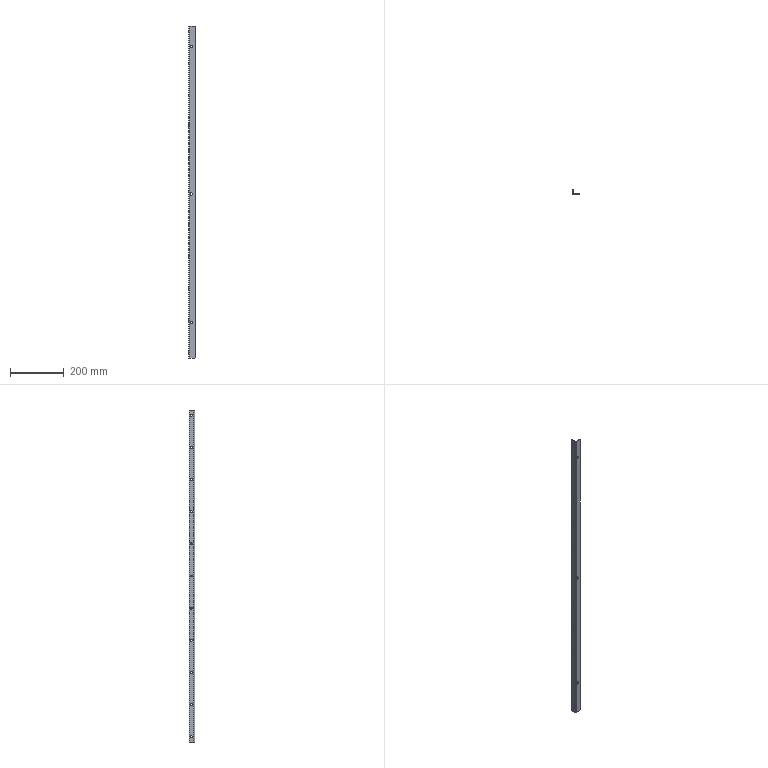Part | NX | features solid 2 | 1 solid | 40 faces | box 25 x 20 x 1240 mm | volume 102183 mm3 | cylinder 30 | plane 10 | commonest cylinder face diameters 7 x22 9.2 x6 4 x1 8 x1
STEP:
#1=CARTESIAN_POINT('',(652.,2.,1242.5));
#2=VERTEX_POINT('',#1);
#3=CARTESIAN_POINT('',(655.,2.,1239.5));
#4=VERTEX_POINT('',#3);
#5=CARTESIAN_POINT('',(655.,2.,1239.5));
#6=DIRECTION('',(0.7071,0.,-0.7071));
#7=VECTOR('',#6,1000.);
#8=LINE('',#5,#7);
#9=EDGE_CURVE('',#2,#4,#8,.T.);
#10=ORIENTED_EDGE('',*,*,#9,.F.);
#11=CARTESIAN_POINT('',(652.,0.,1242.5));
#12=VERTEX_POINT('',#11);
#13=CARTESIAN_POINT('',(652.,0.,1242.5));
#14=DIRECTION('',(0.,1.,0.));
#15=VECTOR('',#14,1000.);
#16=LINE('',#13,#15);
#17=EDGE_CURVE('',#12,#2,#16,.T.);
#18=ORIENTED_EDGE('',*,*,#17,.F.);
#19=CARTESIAN_POINT('',(655.,0.,1239.5));
#20=VERTEX_POINT('',#19);
#21=CARTESIAN_POINT('',(641.,0.,1253.5));
#22=DIRECTION('',(-0.7071,0.,0.7071));
#23=VECTOR('',#22,1000.);
#24=LINE('',#21,#23);
#25=EDGE_CURVE('',#20,#12,#24,.T.);
#26=ORIENTED_EDGE('',*,*,#25,.F.);
#27=CARTESIAN_POINT('',(655.,0.,1239.5));
#28=DIRECTION('',(0.,-1.,0.));
#29=VECTOR('',#28,1000.);
#30=LINE('',#27,#29);
#31=EDGE_CURVE('',#4,#20,#30,.T.);
#32=ORIENTED_EDGE('',*,*,#31,.F.);
#33=EDGE_LOOP('',(#10,#18,#26,#32));
#34=FACE_BOUND('',#33,.T.);
#35=CARTESIAN_POINT('',(655.,0.,1239.5));
#36=DIRECTION('',(-0.7071,0.,-0.7071));
#37=DIRECTION('',(-0.7071,0.,0.7071));
#38=AXIS2_PLACEMENT_3D('',#35,#36,#37);
#39=PLANE('',#38);
#40=ADVANCED_FACE('',(#34),#39,.F.);
#41=CARTESIAN_POINT('',(655.,2.,5.5));
#42=VERTEX_POINT('',#41);
#43=CARTESIAN_POINT('',(652.,2.,2.5));
#44=VERTEX_POINT('',#43);
#45=CARTESIAN_POINT('',(652.,2.,2.5));
#46=DIRECTION('',(-0.7071,0.,-0.7071));
#47=VECTOR('',#46,1000.);
#48=LINE('',#45,#47);
#49=EDGE_CURVE('',#42,#44,#48,.T.);
#50=ORIENTED_EDGE('',*,*,#49,.F.);
#51=CARTESIAN_POINT('',(655.,0.,5.5));
#52=VERTEX_POINT('',#51);
#53=CARTESIAN_POINT('',(655.,0.,5.5));
#54=DIRECTION('',(0.,1.,0.));
#55=VECTOR('',#54,1000.);
#56=LINE('',#53,#55);
#57=EDGE_CURVE('',#52,#42,#56,.T.);
#58=ORIENTED_EDGE('',*,*,#57,.F.);
#59=CARTESIAN_POINT('',(652.,0.,2.5));
#60=VERTEX_POINT('',#59);
#61=CARTESIAN_POINT('',(1261.,0.,611.5));
#62=DIRECTION('',(0.7071,0.,0.7071));
#63=VECTOR('',#62,1000.);
#64=LINE('',#61,#63);
#65=EDGE_CURVE('',#60,#52,#64,.T.);
#66=ORIENTED_EDGE('',*,*,#65,.F.);
#67=CARTESIAN_POINT('',(652.,0.,2.5));
#68=DIRECTION('',(0.,-1.,0.));
#69=VECTOR('',#68,1000.);
#70=LINE('',#67,#69);
#71=EDGE_CURVE('',#44,#60,#70,.T.);
#72=ORIENTED_EDGE('',*,*,#71,.F.);
#73=EDGE_LOOP('',(#50,#58,#66,#72));
#74=FACE_BOUND('',#73,.T.);
#75=CARTESIAN_POINT('',(652.,0.,2.5));
#76=DIRECTION('',(0.7071,0.,-0.7071));
#77=DIRECTION('',(0.,-1.,0.));
#78=AXIS2_PLACEMENT_3D('',#75,#76,#77);
#79=PLANE('',#78);
#80=ADVANCED_FACE('',(#74),#79,.T.);
#81=CARTESIAN_POINT('',(632.,9.,1222.5));
#82=VERTEX_POINT('',#81);
#83=CARTESIAN_POINT('',(630.,9.,1222.5));
#84=VERTEX_POINT('',#83);
#85=CARTESIAN_POINT('',(-608.413,9.,1222.5));
#86=DIRECTION('',(1.,0.,0.));
#87=VECTOR('',#86,1000.);
#88=LINE('',#85,#87);
#89=EDGE_CURVE('',#82,#84,#88,.F.);
#90=ORIENTED_EDGE('',*,*,#89,.T.);
#91=CARTESIAN_POINT('',(630.,16.,1222.5));
#92=VERTEX_POINT('',#91);
#93=CARTESIAN_POINT('',(630.,12.5,1222.5));
#94=DIRECTION('',(1.,0.,0.));
#95=DIRECTION('',(0.,1.,0.));
#96=AXIS2_PLACEMENT_3D('',#93,#94,#95);
#97=CIRCLE('',#96,3.5);
#98=EDGE_CURVE('',#92,#84,#97,.T.);
#99=ORIENTED_EDGE('',*,*,#98,.F.);
#100=CARTESIAN_POINT('',(632.,16.,1222.5));
#101=VERTEX_POINT('',#100);
#102=CARTESIAN_POINT('',(-608.413,16.,1222.5));
#103=DIRECTION('',(1.,0.,0.));
#104=VECTOR('',#103,1000.);
#105=LINE('',#102,#104);
#106=EDGE_CURVE('',#92,#101,#105,.T.);
#107=ORIENTED_EDGE('',*,*,#106,.T.);
#108=CARTESIAN_POINT('',(632.,12.5,1222.5));
#109=DIRECTION('',(1.,0.,0.));
#110=DIRECTION('',(0.,0.,-1.));
#111=AXIS2_PLACEMENT_3D('',#108,#109,#110);
#112=CIRCLE('',#111,3.5);
#113=EDGE_CURVE('',#101,#82,#112,.T.);
#114=ORIENTED_EDGE('',*,*,#113,.T.);
#115=EDGE_LOOP('',(#90,#99,#107,#114));
#116=FACE_BOUND('',#115,.T.);
#117=CARTESIAN_POINT('',(-608.413,12.5,1222.5));
#118=DIRECTION('',(1.,0.,0.));
#119=DIRECTION('',(0.,1.,0.));
#120=AXIS2_PLACEMENT_3D('',#117,#118,#119);
#121=CYLINDRICAL_SURFACE('',#120,3.5);
#122=ADVANCED_FACE('',(#116),#121,.F.);
#123=CARTESIAN_POINT('',(632.,9.,1102.5));
#124=VERTEX_POINT('',#123);
#125=CARTESIAN_POINT('',(630.,9.,1102.5));
#126=VERTEX_POINT('',#125);
#127=CARTESIAN_POINT('',(-608.413,9.,1102.5));
#128=DIRECTION('',(1.,0.,0.));
#129=VECTOR('',#128,1000.);
#130=LINE('',#127,#129);
#131=EDGE_CURVE('',#124,#126,#130,.F.);
#132=ORIENTED_EDGE('',*,*,#131,.T.);
#133=CARTESIAN_POINT('',(630.,16.,1102.5));
#134=VERTEX_POINT('',#133);
#135=CARTESIAN_POINT('',(630.,12.5,1102.5));
#136=DIRECTION('',(1.,0.,0.));
#137=DIRECTION('',(0.,1.,0.));
#138=AXIS2_PLACEMENT_3D('',#135,#136,#137);
#139=CIRCLE('',#138,3.5);
#140=EDGE_CURVE('',#134,#126,#139,.T.);
#141=ORIENTED_EDGE('',*,*,#140,.F.);
#142=CARTESIAN_POINT('',(632.,16.,1102.5));
#143=VERTEX_POINT('',#142);
#144=CARTESIAN_POINT('',(-608.413,16.,1102.5));
#145=DIRECTION('',(1.,0.,0.));
#146=VECTOR('',#145,1000.);
#147=LINE('',#144,#146);
#148=EDGE_CURVE('',#134,#143,#147,.T.);
#149=ORIENTED_EDGE('',*,*,#148,.T.);
#150=CARTESIAN_POINT('',(632.,12.5,1102.5));
#151=DIRECTION('',(1.,0.,0.));
#152=DIRECTION('',(0.,0.,-1.));
#153=AXIS2_PLACEMENT_3D('',#150,#151,#152);
#154=CIRCLE('',#153,3.5);
#155=EDGE_CURVE('',#143,#124,#154,.T.);
#156=ORIENTED_EDGE('',*,*,#155,.T.);
#157=EDGE_LOOP('',(#132,#141,#149,#156));
#158=FACE_BOUND('',#157,.T.);
#159=CARTESIAN_POINT('',(-608.413,12.5,1102.5));
#160=DIRECTION('',(1.,0.,0.));
#161=DIRECTION('',(0.,1.,0.));
#162=AXIS2_PLACEMENT_3D('',#159,#160,#161);
#163=CYLINDRICAL_SURFACE('',#162,3.5);
#164=ADVANCED_FACE('',(#158),#163,.F.);
#165=CARTESIAN_POINT('',(630.,9.,982.5));
#166=VERTEX_POINT('',#165);
#167=CARTESIAN_POINT('',(632.,9.,982.5));
#168=VERTEX_POINT('',#167);
#169=CARTESIAN_POINT('',(-608.413,9.,982.5));
#170=DIRECTION('',(1.,0.,0.));
#171=VECTOR('',#170,1000.);
#172=LINE('',#169,#171);
#173=EDGE_CURVE('',#166,#168,#172,.T.);
#174=ORIENTED_EDGE('',*,*,#173,.F.);
#175=CARTESIAN_POINT('',(630.,16.,982.5));
#176=VERTEX_POINT('',#175);
#177=CARTESIAN_POINT('',(630.,12.5,982.5));
#178=DIRECTION('',(1.,0.,0.));
#179=DIRECTION('',(0.,1.,0.));
#180=AXIS2_PLACEMENT_3D('',#177,#178,#179);
#181=CIRCLE('',#180,3.5);
#182=EDGE_CURVE('',#176,#166,#181,.T.);
#183=ORIENTED_EDGE('',*,*,#182,.F.);
#184=CARTESIAN_POINT('',(632.,16.,982.5));
#185=VERTEX_POINT('',#184);
#186=CARTESIAN_POINT('',(-608.413,16.,982.5));
#187=DIRECTION('',(1.,0.,0.));
#188=VECTOR('',#187,1000.);
#189=LINE('',#186,#188);
#190=EDGE_CURVE('',#185,#176,#189,.F.);
#191=ORIENTED_EDGE('',*,*,#190,.F.);
#192=CARTESIAN_POINT('',(632.,12.5,982.5));
#193=DIRECTION('',(1.,0.,0.));
#194=DIRECTION('',(0.,0.,-1.));
#195=AXIS2_PLACEMENT_3D('',#192,#193,#194);
#196=CIRCLE('',#195,3.5);
#197=EDGE_CURVE('',#185,#168,#196,.T.);
#198=ORIENTED_EDGE('',*,*,#197,.T.);
#199=EDGE_LOOP('',(#174,#183,#191,#198));
#200=FACE_BOUND('',#199,.T.);
#201=CARTESIAN_POINT('',(-608.413,12.5,982.5));
#202=DIRECTION('',(1.,0.,0.));
#203=DIRECTION('',(0.,1.,0.));
#204=AXIS2_PLACEMENT_3D('',#201,#202,#203);
#205=CYLINDRICAL_SURFACE('',#204,3.5);
#206=ADVANCED_FACE('',(#200),#205,.F.);
#207=CARTESIAN_POINT('',(632.,9.,22.5));
#208=VERTEX_POINT('',#207);
#209=CARTESIAN_POINT('',(630.,9.,22.5));
#210=VERTEX_POINT('',#209);
#211=CARTESIAN_POINT('',(-608.413,9.,22.5));
#212=DIRECTION('',(1.,0.,0.));
#213=VECTOR('',#212,1000.);
#214=LINE('',#211,#213);
#215=EDGE_CURVE('',#208,#210,#214,.F.);
#216=ORIENTED_EDGE('',*,*,#215,.T.);
#217=CARTESIAN_POINT('',(630.,16.,22.5));
#218=VERTEX_POINT('',#217);
#219=CARTESIAN_POINT('',(630.,12.5,22.5));
#220=DIRECTION('',(1.,0.,0.));
#221=DIRECTION('',(0.,1.,0.));
#222=AXIS2_PLACEMENT_3D('',#219,#220,#221);
#223=CIRCLE('',#222,3.5);
#224=EDGE_CURVE('',#218,#210,#223,.T.);
#225=ORIENTED_EDGE('',*,*,#224,.F.);
#226=CARTESIAN_POINT('',(632.,16.,22.5));
#227=VERTEX_POINT('',#226);
#228=CARTESIAN_POINT('',(-608.413,16.,22.5));
#229=DIRECTION('',(1.,0.,0.));
#230=VECTOR('',#229,1000.);
#231=LINE('',#228,#230);
#232=EDGE_CURVE('',#218,#227,#231,.T.);
#233=ORIENTED_EDGE('',*,*,#232,.T.);
#234=CARTESIAN_POINT('',(632.,12.5,22.5));
#235=DIRECTION('',(1.,0.,0.));
#236=DIRECTION('',(0.,0.,-1.));
#237=AXIS2_PLACEMENT_3D('',#234,#235,#236);
#238=CIRCLE('',#237,3.5);
#239=EDGE_CURVE('',#227,#208,#238,.T.);
#240=ORIENTED_EDGE('',*,*,#239,.T.);
#241=EDGE_LOOP('',(#216,#225,#233,#240));
#242=FACE_BOUND('',#241,.T.);
#243=CARTESIAN_POINT('',(-608.413,12.5,22.5));
#244=DIRECTION('',(1.,0.,0.));
#245=DIRECTION('',(0.,1.,0.));
#246=AXIS2_PLACEMENT_3D('',#243,#244,#245);
#247=CYLINDRICAL_SURFACE('',#246,3.5);
#248=ADVANCED_FACE('',(#242),#247,.F.);
#249=CARTESIAN_POINT('',(630.,9.,142.5));
#250=VERTEX_POINT('',#249);
#251=CARTESIAN_POINT('',(632.,9.,142.5));
#252=VERTEX_POINT('',#251);
#253=CARTESIAN_POINT('',(-608.413,9.,142.5));
#254=DIRECTION('',(1.,0.,0.));
#255=VECTOR('',#254,1000.);
#256=LINE('',#253,#255);
#257=EDGE_CURVE('',#250,#252,#256,.T.);
#258=ORIENTED_EDGE('',*,*,#257,.F.);
#259=CARTESIAN_POINT('',(630.,16.,142.5));
#260=VERTEX_POINT('',#259);
#261=CARTESIAN_POINT('',(630.,12.5,142.5));
#262=DIRECTION('',(1.,0.,0.));
#263=DIRECTION('',(0.,1.,0.));
#264=AXIS2_PLACEMENT_3D('',#261,#262,#263);
#265=CIRCLE('',#264,3.5);
#266=EDGE_CURVE('',#260,#250,#265,.T.);
#267=ORIENTED_EDGE('',*,*,#266,.F.);
#268=CARTESIAN_POINT('',(632.,16.,142.5));
#269=VERTEX_POINT('',#268);
#270=CARTESIAN_POINT('',(-608.413,16.,142.5));
#271=DIRECTION('',(1.,0.,0.));
#272=VECTOR('',#271,1000.);
#273=LINE('',#270,#272);
#274=EDGE_CURVE('',#269,#260,#273,.F.);
#275=ORIENTED_EDGE('',*,*,#274,.F.);
#276=CARTESIAN_POINT('',(632.,12.5,142.5));
#277=DIRECTION('',(1.,0.,0.));
#278=DIRECTION('',(0.,0.,-1.));
#279=AXIS2_PLACEMENT_3D('',#276,#277,#278);
#280=CIRCLE('',#279,3.5);
#281=EDGE_CURVE('',#269,#252,#280,.T.);
#282=ORIENTED_EDGE('',*,*,#281,.T.);
#283=EDGE_LOOP('',(#258,#267,#275,#282));
#284=FACE_BOUND('',#283,.T.);
#285=CARTESIAN_POINT('',(-608.413,12.5,142.5));
#286=DIRECTION('',(1.,0.,0.));
#287=DIRECTION('',(0.,1.,0.));
#288=AXIS2_PLACEMENT_3D('',#285,#286,#287);
#289=CYLINDRICAL_SURFACE('',#288,3.5);
#290=ADVANCED_FACE('',(#284),#289,.F.);
#291=CARTESIAN_POINT('',(632.,9.,862.5));
#292=VERTEX_POINT('',#291);
#293=CARTESIAN_POINT('',(630.,9.,862.5));
#294=VERTEX_POINT('',#293);
#295=CARTESIAN_POINT('',(-608.413,9.,862.5));
#296=DIRECTION('',(1.,0.,0.));
#297=VECTOR('',#296,1000.);
#298=LINE('',#295,#297);
#299=EDGE_CURVE('',#292,#294,#298,.F.);
#300=ORIENTED_EDGE('',*,*,#299,.T.);
#301=CARTESIAN_POINT('',(630.,16.,862.5));
#302=VERTEX_POINT('',#301);
#303=CARTESIAN_POINT('',(630.,12.5,862.5));
#304=DIRECTION('',(1.,0.,0.));
#305=DIRECTION('',(0.,1.,0.));
#306=AXIS2_PLACEMENT_3D('',#303,#304,#305);
#307=CIRCLE('',#306,3.5);
#308=EDGE_CURVE('',#302,#294,#307,.T.);
#309=ORIENTED_EDGE('',*,*,#308,.F.);
#310=CARTESIAN_POINT('',(632.,16.,862.5));
#311=VERTEX_POINT('',#310);
#312=CARTESIAN_POINT('',(-608.413,16.,862.5));
#313=DIRECTION('',(1.,0.,0.));
#314=VECTOR('',#313,1000.);
#315=LINE('',#312,#314);
#316=EDGE_CURVE('',#302,#311,#315,.T.);
#317=ORIENTED_EDGE('',*,*,#316,.T.);
#318=CARTESIAN_POINT('',(632.,12.5,862.5));
#319=DIRECTION('',(1.,0.,0.));
#320=DIRECTION('',(0.,0.,-1.));
#321=AXIS2_PLACEMENT_3D('',#318,#319,#320);
#322=CIRCLE('',#321,3.5);
#323=EDGE_CURVE('',#311,#292,#322,.T.);
#324=ORIENTED_EDGE('',*,*,#323,.T.);
#325=EDGE_LOOP('',(#300,#309,#317,#324));
#326=FACE_BOUND('',#325,.T.);
#327=CARTESIAN_POINT('',(-608.413,12.5,862.5));
#328=DIRECTION('',(1.,0.,0.));
#329=DIRECTION('',(0.,1.,0.));
#330=AXIS2_PLACEMENT_3D('',#327,#328,#329);
#331=CYLINDRICAL_SURFACE('',#330,3.5);
#332=ADVANCED_FACE('',(#326),#331,.F.);
#333=CARTESIAN_POINT('',(630.,9.,742.5));
#334=VERTEX_POINT('',#333);
#335=CARTESIAN_POINT('',(632.,9.,742.5));
#336=VERTEX_POINT('',#335);
#337=CARTESIAN_POINT('',(-608.413,9.,742.5));
#338=DIRECTION('',(1.,0.,0.));
#339=VECTOR('',#338,1000.);
#340=LINE('',#337,#339);
#341=EDGE_CURVE('',#334,#336,#340,.T.);
#342=ORIENTED_EDGE('',*,*,#341,.F.);
#343=CARTESIAN_POINT('',(630.,16.,742.5));
#344=VERTEX_POINT('',#343);
#345=CARTESIAN_POINT('',(630.,12.5,742.5));
#346=DIRECTION('',(1.,0.,0.));
#347=DIRECTION('',(0.,1.,0.));
#348=AXIS2_PLACEMENT_3D('',#345,#346,#347);
#349=CIRCLE('',#348,3.5);
#350=EDGE_CURVE('',#344,#334,#349,.T.);
#351=ORIENTED_EDGE('',*,*,#350,.F.);
#352=CARTESIAN_POINT('',(632.,16.,742.5));
#353=VERTEX_POINT('',#352);
#354=CARTESIAN_POINT('',(-608.413,16.,742.5));
#355=DIRECTION('',(1.,0.,0.));
#356=VECTOR('',#355,1000.);
#357=LINE('',#354,#356);
#358=EDGE_CURVE('',#353,#344,#357,.F.);
#359=ORIENTED_EDGE('',*,*,#358,.F.);
#360=CARTESIAN_POINT('',(632.,12.5,742.5));
#361=DIRECTION('',(1.,0.,0.));
#362=DIRECTION('',(0.,0.,-1.));
#363=AXIS2_PLACEMENT_3D('',#360,#361,#362);
#364=CIRCLE('',#363,3.5);
#365=EDGE_CURVE('',#353,#336,#364,.T.);
#366=ORIENTED_EDGE('',*,*,#365,.T.);
#367=EDGE_LOOP('',(#342,#351,#359,#366));
#368=FACE_BOUND('',#367,.T.);
#369=CARTESIAN_POINT('',(-608.413,12.5,742.5));
#370=DIRECTION('',(1.,0.,0.));
#371=DIRECTION('',(0.,1.,0.));
#372=AXIS2_PLACEMENT_3D('',#369,#370,#371);
#373=CYLINDRICAL_SURFACE('',#372,3.5);
#374=ADVANCED_FACE('',(#368),#373,.F.);
#375=CARTESIAN_POINT('',(632.,9.,622.5));
#376=VERTEX_POINT('',#375);
#377=CARTESIAN_POINT('',(630.,9.,622.5));
#378=VERTEX_POINT('',#377);
#379=CARTESIAN_POINT('',(-608.413,9.,622.5));
#380=DIRECTION('',(1.,0.,0.));
#381=VECTOR('',#380,1000.);
#382=LINE('',#379,#381);
#383=EDGE_CURVE('',#376,#378,#382,.F.);
#384=ORIENTED_EDGE('',*,*,#383,.T.);
#385=CARTESIAN_POINT('',(630.,16.,622.5));
#386=VERTEX_POINT('',#385);
#387=CARTESIAN_POINT('',(630.,12.5,622.5));
#388=DIRECTION('',(1.,0.,0.));
#389=DIRECTION('',(0.,1.,0.));
#390=AXIS2_PLACEMENT_3D('',#387,#388,#389);
#391=CIRCLE('',#390,3.5);
#392=EDGE_CURVE('',#386,#378,#391,.T.);
#393=ORIENTED_EDGE('',*,*,#392,.F.);
#394=CARTESIAN_POINT('',(632.,16.,622.5));
#395=VERTEX_POINT('',#394);
#396=CARTESIAN_POINT('',(-608.413,16.,622.5));
#397=DIRECTION('',(1.,0.,0.));
#398=VECTOR('',#397,1000.);
#399=LINE('',#396,#398);
#400=EDGE_CURVE('',#386,#395,#399,.T.);
#401=ORIENTED_EDGE('',*,*,#400,.T.);
#402=CARTESIAN_POINT('',(632.,12.5,622.5));
#403=DIRECTION('',(1.,0.,0.));
#404=DIRECTION('',(0.,0.,-1.));
#405=AXIS2_PLACEMENT_3D('',#402,#403,#404);
#406=CIRCLE('',#405,3.5);
#407=EDGE_CURVE('',#395,#376,#406,.T.);
#408=ORIENTED_EDGE('',*,*,#407,.T.);
#409=EDGE_LOOP('',(#384,#393,#401,#408));
#410=FACE_BOUND('',#409,.T.);
#411=CARTESIAN_POINT('',(-608.413,12.5,622.5));
#412=DIRECTION('',(1.,0.,0.));
#413=DIRECTION('',(0.,1.,0.));
#414=AXIS2_PLACEMENT_3D('',#411,#412,#413);
#415=CYLINDRICAL_SURFACE('',#414,3.5);
#416=ADVANCED_FACE('',(#410),#415,.F.);
#417=CARTESIAN_POINT('',(630.,9.,502.5));
#418=VERTEX_POINT('',#417);
#419=CARTESIAN_POINT('',(632.,9.,502.5));
#420=VERTEX_POINT('',#419);
#421=CARTESIAN_POINT('',(-608.413,9.,502.5));
#422=DIRECTION('',(1.,0.,0.));
#423=VECTOR('',#422,1000.);
#424=LINE('',#421,#423);
#425=EDGE_CURVE('',#418,#420,#424,.T.);
#426=ORIENTED_EDGE('',*,*,#425,.F.);
#427=CARTESIAN_POINT('',(630.,16.,502.5));
#428=VERTEX_POINT('',#427);
#429=CARTESIAN_POINT('',(630.,12.5,502.5));
#430=DIRECTION('',(1.,0.,0.));
#431=DIRECTION('',(0.,1.,0.));
#432=AXIS2_PLACEMENT_3D('',#429,#430,#431);
#433=CIRCLE('',#432,3.5);
#434=EDGE_CURVE('',#428,#418,#433,.T.);
#435=ORIENTED_EDGE('',*,*,#434,.F.);
#436=CARTESIAN_POINT('',(632.,16.,502.5));
#437=VERTEX_POINT('',#436);
#438=CARTESIAN_POINT('',(-608.413,16.,502.5));
#439=DIRECTION('',(1.,0.,0.));
#440=VECTOR('',#439,1000.);
#441=LINE('',#438,#440);
#442=EDGE_CURVE('',#437,#428,#441,.F.);
#443=ORIENTED_EDGE('',*,*,#442,.F.);
#444=CARTESIAN_POINT('',(632.,12.5,502.5));
#445=DIRECTION('',(1.,0.,0.));
#446=DIRECTION('',(0.,0.,-1.));
#447=AXIS2_PLACEMENT_3D('',#444,#445,#446);
#448=CIRCLE('',#447,3.5);
#449=EDGE_CURVE('',#437,#420,#448,.T.);
#450=ORIENTED_EDGE('',*,*,#449,.T.);
#451=EDGE_LOOP('',(#426,#435,#443,#450));
#452=FACE_BOUND('',#451,.T.);
#453=CARTESIAN_POINT('',(-608.413,12.5,502.5));
#454=DIRECTION('',(1.,0.,0.));
#455=DIRECTION('',(0.,1.,0.));
#456=AXIS2_PLACEMENT_3D('',#453,#454,#455);
#457=CYLINDRICAL_SURFACE('',#456,3.5);
#458=ADVANCED_FACE('',(#452),#457,.F.);
#459=CARTESIAN_POINT('',(630.,9.,382.5));
#460=VERTEX_POINT('',#459);
#461=CARTESIAN_POINT('',(632.,9.,382.5));
#462=VERTEX_POINT('',#461);
#463=CARTESIAN_POINT('',(-608.413,9.,382.5));
#464=DIRECTION('',(1.,0.,0.));
#465=VECTOR('',#464,1000.);
#466=LINE('',#463,#465);
#467=EDGE_CURVE('',#460,#462,#466,.T.);
#468=ORIENTED_EDGE('',*,*,#467,.F.);
#469=CARTESIAN_POINT('',(630.,16.,382.5));
#470=VERTEX_POINT('',#469);
#471=CARTESIAN_POINT('',(630.,12.5,382.5));
#472=DIRECTION('',(1.,0.,0.));
#473=DIRECTION('',(0.,1.,0.));
#474=AXIS2_PLACEMENT_3D('',#471,#472,#473);
#475=CIRCLE('',#474,3.5);
#476=EDGE_CURVE('',#470,#460,#475,.T.);
#477=ORIENTED_EDGE('',*,*,#476,.F.);
#478=CARTESIAN_POINT('',(632.,16.,382.5));
#479=VERTEX_POINT('',#478);
#480=CARTESIAN_POINT('',(-608.413,16.,382.5));
#481=DIRECTION('',(1.,0.,0.));
#482=VECTOR('',#481,1000.);
#483=LINE('',#480,#482);
#484=EDGE_CURVE('',#479,#470,#483,.F.);
#485=ORIENTED_EDGE('',*,*,#484,.F.);
#486=CARTESIAN_POINT('',(632.,12.5,382.5));
#487=DIRECTION('',(1.,0.,0.));
#488=DIRECTION('',(0.,0.,-1.));
#489=AXIS2_PLACEMENT_3D('',#486,#487,#488);
#490=CIRCLE('',#489,3.5);
#491=EDGE_CURVE('',#479,#462,#490,.T.);
#492=ORIENTED_EDGE('',*,*,#491,.T.);
#493=EDGE_LOOP('',(#468,#477,#485,#492));
#494=FACE_BOUND('',#493,.T.);
#495=CARTESIAN_POINT('',(-608.413,12.5,382.5));
#496=DIRECTION('',(1.,0.,0.));
#497=DIRECTION('',(0.,1.,0.));
#498=AXIS2_PLACEMENT_3D('',#495,#496,#497);
#499=CYLINDRICAL_SURFACE('',#498,3.5);
#500=ADVANCED_FACE('',(#494),#499,.F.);
#501=CARTESIAN_POINT('',(630.,9.,262.5));
#502=VERTEX_POINT('',#501);
#503=CARTESIAN_POINT('',(632.,9.,262.5));
#504=VERTEX_POINT('',#503);
#505=CARTESIAN_POINT('',(-608.413,9.,262.5));
#506=DIRECTION('',(1.,0.,0.));
#507=VECTOR('',#506,1000.);
#508=LINE('',#505,#507);
#509=EDGE_CURVE('',#502,#504,#508,.T.);
#510=ORIENTED_EDGE('',*,*,#509,.F.);
#511=CARTESIAN_POINT('',(630.,16.,262.5));
#512=VERTEX_POINT('',#511);
#513=CARTESIAN_POINT('',(630.,12.5,262.5));
#514=DIRECTION('',(1.,0.,0.));
#515=DIRECTION('',(0.,1.,0.));
#516=AXIS2_PLACEMENT_3D('',#513,#514,#515);
#517=CIRCLE('',#516,3.5);
#518=EDGE_CURVE('',#512,#502,#517,.T.);
#519=ORIENTED_EDGE('',*,*,#518,.F.);
#520=CARTESIAN_POINT('',(632.,16.,262.5));
#521=VERTEX_POINT('',#520);
#522=CARTESIAN_POINT('',(-608.413,16.,262.5));
#523=DIRECTION('',(1.,0.,0.));
#524=VECTOR('',#523,1000.);
#525=LINE('',#522,#524);
#526=EDGE_CURVE('',#521,#512,#525,.F.);
#527=ORIENTED_EDGE('',*,*,#526,.F.);
#528=CARTESIAN_POINT('',(632.,12.5,262.5));
#529=DIRECTION('',(1.,0.,0.));
#530=DIRECTION('',(0.,0.,-1.));
#531=AXIS2_PLACEMENT_3D('',#528,#529,#530);
#532=CIRCLE('',#531,3.5);
#533=EDGE_CURVE('',#521,#504,#532,.T.);
#534=ORIENTED_EDGE('',*,*,#533,.T.);
#535=EDGE_LOOP('',(#510,#519,#527,#534));
#536=FACE_BOUND('',#535,.T.);
#537=CARTESIAN_POINT('',(-608.413,12.5,262.5));
#538=DIRECTION('',(1.,0.,0.));
#539=DIRECTION('',(0.,1.,0.));
#540=AXIS2_PLACEMENT_3D('',#537,#538,#539);
#541=CYLINDRICAL_SURFACE('',#540,3.5);
#542=ADVANCED_FACE('',(#536),#541,.F.);
#543=CARTESIAN_POINT('',(640.,2.,619.6));
#544=VERTEX_POINT('',#543);
#545=CARTESIAN_POINT('',(640.,0.,619.6));
#546=VERTEX_POINT('',#545);
#547=CARTESIAN_POINT('',(640.,1240.413,619.6));
#548=DIRECTION('',(0.,-1.,0.));
#549=VECTOR('',#548,1000.);
#550=LINE('',#547,#549);
#551=EDGE_CURVE('',#544,#546,#550,.T.);
#552=ORIENTED_EDGE('',*,*,#551,.F.);
#553=CARTESIAN_POINT('',(640.,2.,610.4));
#554=VERTEX_POINT('',#553);
#555=CARTESIAN_POINT('',(640.,2.,615.));
#556=DIRECTION('',(0.,-1.,0.));
#557=DIRECTION('',(0.,0.,-1.));
#558=AXIS2_PLACEMENT_3D('',#555,#556,#557);
#559=CIRCLE('',#558,4.6);
#560=EDGE_CURVE('',#554,#544,#559,.T.);
#561=ORIENTED_EDGE('',*,*,#560,.F.);
#562=CARTESIAN_POINT('',(640.,0.,610.4));
#563=VERTEX_POINT('',#562);
#564=CARTESIAN_POINT('',(640.,1240.413,610.4));
#565=DIRECTION('',(0.,-1.,0.));
#566=VECTOR('',#565,1000.);
#567=LINE('',#564,#566);
#568=EDGE_CURVE('',#563,#554,#567,.F.);
#569=ORIENTED_EDGE('',*,*,#568,.F.);
#570=CARTESIAN_POINT('',(640.,0.,615.));
#571=DIRECTION('',(0.,-1.,0.));
#572=DIRECTION('',(0.,0.,1.));
#573=AXIS2_PLACEMENT_3D('',#570,#571,#572);
#574=CIRCLE('',#573,4.6);
#575=EDGE_CURVE('',#563,#546,#574,.T.);
#576=ORIENTED_EDGE('',*,*,#575,.T.);
#577=EDGE_LOOP('',(#552,#561,#569,#576));
#578=FACE_BOUND('',#577,.T.);
#579=CARTESIAN_POINT('',(640.,1240.413,615.));
#580=DIRECTION('',(0.,-1.,0.));
#581=DIRECTION('',(0.,0.,-1.));
#582=AXIS2_PLACEMENT_3D('',#579,#580,#581);
#583=CYLINDRICAL_SURFACE('',#582,4.6);
#584=ADVANCED_FACE('',(#578),#583,.F.);
#585=CARTESIAN_POINT('',(640.,2.,1169.6));
#586=VERTEX_POINT('',#585);
#587=CARTESIAN_POINT('',(640.,0.,1169.6));
#588=VERTEX_POINT('',#587);
#589=CARTESIAN_POINT('',(640.,1240.413,1169.6));
#590=DIRECTION('',(0.,-1.,0.));
#591=VECTOR('',#590,1000.);
#592=LINE('',#589,#591);
#593=EDGE_CURVE('',#586,#588,#592,.T.);
#594=ORIENTED_EDGE('',*,*,#593,.F.);
#595=CARTESIAN_POINT('',(640.,2.,1160.4));
#596=VERTEX_POINT('',#595);
#597=CARTESIAN_POINT('',(640.,2.,1165.));
#598=DIRECTION('',(0.,-1.,0.));
#599=DIRECTION('',(0.,0.,-1.));
#600=AXIS2_PLACEMENT_3D('',#597,#598,#599);
#601=CIRCLE('',#600,4.6);
#602=EDGE_CURVE('',#596,#586,#601,.T.);
#603=ORIENTED_EDGE('',*,*,#602,.F.);
#604=CARTESIAN_POINT('',(640.,0.,1160.4));
#605=VERTEX_POINT('',#604);
#606=CARTESIAN_POINT('',(640.,1240.413,1160.4));
#607=DIRECTION('',(0.,-1.,0.));
#608=VECTOR('',#607,1000.);
#609=LINE('',#606,#608);
#610=EDGE_CURVE('',#605,#596,#609,.F.);
#611=ORIENTED_EDGE('',*,*,#610,.F.);
#612=CARTESIAN_POINT('',(640.,0.,1165.));
#613=DIRECTION('',(0.,-1.,0.));
#614=DIRECTION('',(0.,0.,1.));
#615=AXIS2_PLACEMENT_3D('',#612,#613,#614);
#616=CIRCLE('',#615,4.6);
#617=EDGE_CURVE('',#605,#588,#616,.T.);
#618=ORIENTED_EDGE('',*,*,#617,.T.);
#619=EDGE_LOOP('',(#594,#603,#611,#618));
#620=FACE_BOUND('',#619,.T.);
#621=CARTESIAN_POINT('',(640.,1240.413,1165.));
#622=DIRECTION('',(0.,-1.,0.));
#623=DIRECTION('',(0.,0.,-1.));
#624=AXIS2_PLACEMENT_3D('',#621,#622,#623);
#625=CYLINDRICAL_SURFACE('',#624,4.6);
#626=ADVANCED_FACE('',(#620),#625,.F.);
#627=CARTESIAN_POINT('',(640.,2.,139.6));
#628=VERTEX_POINT('',#627);
#629=CARTESIAN_POINT('',(640.,0.,139.6));
#630=VERTEX_POINT('',#629);
#631=CARTESIAN_POINT('',(640.,1240.413,139.6));
#632=DIRECTION('',(0.,-1.,0.));
#633=VECTOR('',#632,1000.);
#634=LINE('',#631,#633);
#635=EDGE_CURVE('',#628,#630,#634,.T.);
#636=ORIENTED_EDGE('',*,*,#635,.F.);
#637=CARTESIAN_POINT('',(640.,2.,130.4));
#638=VERTEX_POINT('',#637);
#639=CARTESIAN_POINT('',(640.,2.,135.));
#640=DIRECTION('',(0.,-1.,0.));
#641=DIRECTION('',(0.,0.,-1.));
#642=AXIS2_PLACEMENT_3D('',#639,#640,#641);
#643=CIRCLE('',#642,4.6);
#644=EDGE_CURVE('',#638,#628,#643,.T.);
#645=ORIENTED_EDGE('',*,*,#644,.F.);
#646=CARTESIAN_POINT('',(640.,0.,130.4));
#647=VERTEX_POINT('',#646);
#648=CARTESIAN_POINT('',(640.,1240.413,130.4));
#649=DIRECTION('',(0.,-1.,0.));
#650=VECTOR('',#649,1000.);
#651=LINE('',#648,#650);
#652=EDGE_CURVE('',#647,#638,#651,.F.);
#653=ORIENTED_EDGE('',*,*,#652,.F.);
#654=CARTESIAN_POINT('',(640.,0.,135.));
#655=DIRECTION('',(0.,-1.,0.));
#656=DIRECTION('',(0.,0.,1.));
#657=AXIS2_PLACEMENT_3D('',#654,#655,#656);
#658=CIRCLE('',#657,4.6);
#659=EDGE_CURVE('',#647,#630,#658,.T.);
#660=ORIENTED_EDGE('',*,*,#659,.T.);
#661=EDGE_LOOP('',(#636,#645,#653,#660));
#662=FACE_BOUND('',#661,.T.);
#663=CARTESIAN_POINT('',(640.,1240.413,135.));
#664=DIRECTION('',(0.,-1.,0.));
#665=DIRECTION('',(0.,0.,-1.));
#666=AXIS2_PLACEMENT_3D('',#663,#664,#665);
#667=CYLINDRICAL_SURFACE('',#666,4.6);
#668=ADVANCED_FACE('',(#662),#667,.F.);
#669=CARTESIAN_POINT('',(634.,2.,1242.5));
#670=VERTEX_POINT('',#669);
#671=CARTESIAN_POINT('',(634.,2.,2.5));
#672=VERTEX_POINT('',#671);
#673=CARTESIAN_POINT('',(634.,2.,1242.5));
#674=DIRECTION('',(0.,0.,-1.));
#675=VECTOR('',#674,1000.);
#676=LINE('',#673,#675);
#677=EDGE_CURVE('',#670,#672,#676,.T.);
#678=ORIENTED_EDGE('',*,*,#677,.T.);
#679=CARTESIAN_POINT('',(632.,4.,2.5));
#680=VERTEX_POINT('',#679);
#681=CARTESIAN_POINT('',(634.,4.,2.5));
#682=DIRECTION('',(0.,0.,1.));
#683=DIRECTION('',(0.,1.,0.));
#684=AXIS2_PLACEMENT_3D('',#681,#682,#683);
#685=CIRCLE('',#684,2.);
#686=EDGE_CURVE('',#680,#672,#685,.T.);
#687=ORIENTED_EDGE('',*,*,#686,.F.);
#688=CARTESIAN_POINT('',(632.,4.,1242.5));
#689=VERTEX_POINT('',#688);
#690=CARTESIAN_POINT('',(632.,4.,2.5));
#691=DIRECTION('',(0.,0.,1.));
#692=VECTOR('',#691,1000.);
#693=LINE('',#690,#692);
#694=EDGE_CURVE('',#680,#689,#693,.T.);
#695=ORIENTED_EDGE('',*,*,#694,.T.);
#696=CARTESIAN_POINT('',(634.,4.,1242.5));
#697=DIRECTION('',(0.,0.,1.));
#698=DIRECTION('',(0.,1.,0.));
#699=AXIS2_PLACEMENT_3D('',#696,#697,#698);
#700=CIRCLE('',#699,2.);
#701=EDGE_CURVE('',#689,#670,#700,.T.);
#702=ORIENTED_EDGE('',*,*,#701,.T.);
#703=EDGE_LOOP('',(#678,#687,#695,#702));
#704=FACE_BOUND('',#703,.T.);
#705=CARTESIAN_POINT('',(634.,4.,1242.5));
#706=DIRECTION('',(0.,0.,-1.));
#707=DIRECTION('',(0.,1.,0.));
#708=AXIS2_PLACEMENT_3D('',#705,#706,#707);
#709=CYLINDRICAL_SURFACE('',#708,2.);
#710=ADVANCED_FACE('',(#704),#709,.F.);
#711=CARTESIAN_POINT('',(634.,0.,1242.5));
#712=VERTEX_POINT('',#711);
#713=CARTESIAN_POINT('',(634.,0.,2.5));
#714=VERTEX_POINT('',#713);
#715=CARTESIAN_POINT('',(634.,0.,1242.5));
#716=DIRECTION('',(0.,0.,-1.));
#717=VECTOR('',#716,1000.);
#718=LINE('',#715,#717);
#719=EDGE_CURVE('',#712,#714,#718,.T.);
#720=ORIENTED_EDGE('',*,*,#719,.F.);
#721=CARTESIAN_POINT('',(630.,4.,1242.5));
#722=VERTEX_POINT('',#721);
#723=CARTESIAN_POINT('',(634.,4.,1242.5));
#724=DIRECTION('',(0.,0.,1.));
#725=DIRECTION('',(0.,1.,0.));
#726=AXIS2_PLACEMENT_3D('',#723,#724,#725);
#727=CIRCLE('',#726,4.);
#728=EDGE_CURVE('',#722,#712,#727,.T.);
#729=ORIENTED_EDGE('',*,*,#728,.F.);
#730=CARTESIAN_POINT('',(630.,4.,2.5));
#731=VERTEX_POINT('',#730);
#732=CARTESIAN_POINT('',(630.,4.,2.5));
#733=DIRECTION('',(0.,0.,1.));
#734=VECTOR('',#733,1000.);
#735=LINE('',#732,#734);
#736=EDGE_CURVE('',#731,#722,#735,.T.);
#737=ORIENTED_EDGE('',*,*,#736,.F.);
#738=CARTESIAN_POINT('',(634.,4.,2.5));
#739=DIRECTION('',(0.,0.,1.));
#740=DIRECTION('',(0.,1.,0.));
#741=AXIS2_PLACEMENT_3D('',#738,#739,#740);
#742=CIRCLE('',#741,4.);
#743=EDGE_CURVE('',#731,#714,#742,.T.);
#744=ORIENTED_EDGE('',*,*,#743,.T.);
#745=EDGE_LOOP('',(#720,#729,#737,#744));
#746=FACE_BOUND('',#745,.T.);
#747=CARTESIAN_POINT('',(634.,4.,1242.5));
#748=DIRECTION('',(0.,0.,-1.));
#749=DIRECTION('',(0.,1.,0.));
#750=AXIS2_PLACEMENT_3D('',#747,#748,#749);
#751=CYLINDRICAL_SURFACE('',#750,4.);
#752=ADVANCED_FACE('',(#746),#751,.T.);
#753=ORIENTED_EDGE('',*,*,#533,.F.);
#754=CARTESIAN_POINT('',(632.,12.5,262.5));
#755=DIRECTION('',(1.,0.,0.));
#756=DIRECTION('',(0.,0.,-1.));
#757=AXIS2_PLACEMENT_3D('',#754,#755,#756);
#758=CIRCLE('',#757,3.5);
#759=EDGE_CURVE('',#504,#521,#758,.T.);
#760=ORIENTED_EDGE('',*,*,#759,.F.);
#761=EDGE_LOOP('',(#753,#760));
#762=FACE_BOUND('',#761,.T.);
#763=ORIENTED_EDGE('',*,*,#491,.F.);
#764=CARTESIAN_POINT('',(632.,12.5,382.5));
#765=DIRECTION('',(1.,0.,0.));
#766=DIRECTION('',(0.,0.,-1.));
#767=AXIS2_PLACEMENT_3D('',#764,#765,#766);
#768=CIRCLE('',#767,3.5);
#769=EDGE_CURVE('',#462,#479,#768,.T.);
#770=ORIENTED_EDGE('',*,*,#769,.F.);
#771=EDGE_LOOP('',(#763,#770));
#772=FACE_BOUND('',#771,.T.);
#773=ORIENTED_EDGE('',*,*,#449,.F.);
#774=CARTESIAN_POINT('',(632.,12.5,502.5));
#775=DIRECTION('',(1.,0.,0.));
#776=DIRECTION('',(0.,0.,-1.));
#777=AXIS2_PLACEMENT_3D('',#774,#775,#776);
#778=CIRCLE('',#777,3.5);
#779=EDGE_CURVE('',#420,#437,#778,.T.);
#780=ORIENTED_EDGE('',*,*,#779,.F.);
#781=EDGE_LOOP('',(#773,#780));
#782=FACE_BOUND('',#781,.T.);
#783=ORIENTED_EDGE('',*,*,#407,.F.);
#784=CARTESIAN_POINT('',(632.,12.5,622.5));
#785=DIRECTION('',(1.,0.,0.));
#786=DIRECTION('',(0.,0.,-1.));
#787=AXIS2_PLACEMENT_3D('',#784,#785,#786);
#788=CIRCLE('',#787,3.5);
#789=EDGE_CURVE('',#376,#395,#788,.T.);
#790=ORIENTED_EDGE('',*,*,#789,.F.);
#791=EDGE_LOOP('',(#783,#790));
#792=FACE_BOUND('',#791,.T.);
#793=ORIENTED_EDGE('',*,*,#365,.F.);
#794=CARTESIAN_POINT('',(632.,12.5,742.5));
#795=DIRECTION('',(1.,0.,0.));
#796=DIRECTION('',(0.,0.,-1.));
#797=AXIS2_PLACEMENT_3D('',#794,#795,#796);
#798=CIRCLE('',#797,3.5);
#799=EDGE_CURVE('',#336,#353,#798,.T.);
#800=ORIENTED_EDGE('',*,*,#799,.F.);
#801=EDGE_LOOP('',(#793,#800));
#802=FACE_BOUND('',#801,.T.);
#803=ORIENTED_EDGE('',*,*,#323,.F.);
#804=CARTESIAN_POINT('',(632.,12.5,862.5));
#805=DIRECTION('',(1.,0.,0.));
#806=DIRECTION('',(0.,0.,-1.));
#807=AXIS2_PLACEMENT_3D('',#804,#805,#806);
#808=CIRCLE('',#807,3.5);
#809=EDGE_CURVE('',#292,#311,#808,.T.);
#810=ORIENTED_EDGE('',*,*,#809,.F.);
#811=EDGE_LOOP('',(#803,#810));
#812=FACE_BOUND('',#811,.T.);
#813=ORIENTED_EDGE('',*,*,#281,.F.);
#814=CARTESIAN_POINT('',(632.,12.5,142.5));
#815=DIRECTION('',(1.,0.,0.));
#816=DIRECTION('',(0.,0.,-1.));
#817=AXIS2_PLACEMENT_3D('',#814,#815,#816);
#818=CIRCLE('',#817,3.5);
#819=EDGE_CURVE('',#252,#269,#818,.T.);
#820=ORIENTED_EDGE('',*,*,#819,.F.);
#821=EDGE_LOOP('',(#813,#820));
#822=FACE_BOUND('',#821,.T.);
#823=ORIENTED_EDGE('',*,*,#239,.F.);
#824=CARTESIAN_POINT('',(632.,12.5,22.5));
#825=DIRECTION('',(1.,0.,0.));
#826=DIRECTION('',(0.,0.,-1.));
#827=AXIS2_PLACEMENT_3D('',#824,#825,#826);
#828=CIRCLE('',#827,3.5);
#829=EDGE_CURVE('',#208,#227,#828,.T.);
#830=ORIENTED_EDGE('',*,*,#829,.F.);
#831=EDGE_LOOP('',(#823,#830));
#832=FACE_BOUND('',#831,.T.);
#833=ORIENTED_EDGE('',*,*,#197,.F.);
#834=CARTESIAN_POINT('',(632.,12.5,982.5));
#835=DIRECTION('',(1.,0.,0.));
#836=DIRECTION('',(0.,0.,-1.));
#837=AXIS2_PLACEMENT_3D('',#834,#835,#836);
#838=CIRCLE('',#837,3.5);
#839=EDGE_CURVE('',#168,#185,#838,.T.);
#840=ORIENTED_EDGE('',*,*,#839,.F.);
#841=EDGE_LOOP('',(#833,#840));
#842=FACE_BOUND('',#841,.T.);
#843=ORIENTED_EDGE('',*,*,#155,.F.);
#844=CARTESIAN_POINT('',(632.,12.5,1102.5));
#845=DIRECTION('',(1.,0.,0.));
#846=DIRECTION('',(0.,0.,-1.));
#847=AXIS2_PLACEMENT_3D('',#844,#845,#846);
#848=CIRCLE('',#847,3.5);
#849=EDGE_CURVE('',#124,#143,#848,.T.);
#850=ORIENTED_EDGE('',*,*,#849,.F.);
#851=EDGE_LOOP('',(#843,#850));
#852=FACE_BOUND('',#851,.T.);
#853=ORIENTED_EDGE('',*,*,#113,.F.);
#854=CARTESIAN_POINT('',(632.,12.5,1222.5));
#855=DIRECTION('',(1.,0.,0.));
#856=DIRECTION('',(0.,0.,-1.));
#857=AXIS2_PLACEMENT_3D('',#854,#855,#856);
#858=CIRCLE('',#857,3.5);
#859=EDGE_CURVE('',#82,#101,#858,.T.);
#860=ORIENTED_EDGE('',*,*,#859,.F.);
#861=EDGE_LOOP('',(#853,#860));
#862=FACE_BOUND('',#861,.T.);
#863=CARTESIAN_POINT('',(632.,20.,1242.5));
#864=VERTEX_POINT('',#863);
#865=CARTESIAN_POINT('',(632.,0.,1242.5));
#866=DIRECTION('',(0.,1.,0.));
#867=VECTOR('',#866,1000.);
#868=LINE('',#865,#867);
#869=EDGE_CURVE('',#689,#864,#868,.T.);
#870=ORIENTED_EDGE('',*,*,#869,.F.);
#871=ORIENTED_EDGE('',*,*,#694,.F.);
#872=CARTESIAN_POINT('',(632.,20.,2.5));
#873=VERTEX_POINT('',#872);
#874=CARTESIAN_POINT('',(632.,0.,2.5));
#875=DIRECTION('',(0.,1.,0.));
#876=VECTOR('',#875,1000.);
#877=LINE('',#874,#876);
#878=EDGE_CURVE('',#680,#873,#877,.T.);
#879=ORIENTED_EDGE('',*,*,#878,.T.);
#880=CARTESIAN_POINT('',(632.,20.,2.5));
#881=DIRECTION('',(0.,0.,1.));
#882=VECTOR('',#881,1000.);
#883=LINE('',#880,#882);
#884=EDGE_CURVE('',#873,#864,#883,.T.);
#885=ORIENTED_EDGE('',*,*,#884,.T.);
#886=EDGE_LOOP('',(#870,#871,#879,#885));
#887=FACE_BOUND('',#886,.T.);
#888=CARTESIAN_POINT('',(632.,0.,2.5));
#889=DIRECTION('',(1.,0.,0.));
#890=DIRECTION('',(0.,-1.,0.));
#891=AXIS2_PLACEMENT_3D('',#888,#889,#890);
#892=PLANE('',#891);
#893=ADVANCED_FACE('',(#762,#772,#782,#792,#802,#812,#822,#832,#842,#852,#862,#887),#892,.T.);
#894=ORIENTED_EDGE('',*,*,#518,.T.);
#895=CARTESIAN_POINT('',(630.,12.5,262.5));
#896=DIRECTION('',(1.,0.,0.));
#897=DIRECTION('',(0.,1.,0.));
#898=AXIS2_PLACEMENT_3D('',#895,#896,#897);
#899=CIRCLE('',#898,3.5);
#900=EDGE_CURVE('',#502,#512,#899,.T.);
#901=ORIENTED_EDGE('',*,*,#900,.T.);
#902=EDGE_LOOP('',(#894,#901));
#903=FACE_BOUND('',#902,.T.);
#904=ORIENTED_EDGE('',*,*,#476,.T.);
#905=CARTESIAN_POINT('',(630.,12.5,382.5));
#906=DIRECTION('',(1.,0.,0.));
#907=DIRECTION('',(0.,1.,0.));
#908=AXIS2_PLACEMENT_3D('',#905,#906,#907);
#909=CIRCLE('',#908,3.5);
#910=EDGE_CURVE('',#460,#470,#909,.T.);
#911=ORIENTED_EDGE('',*,*,#910,.T.);
#912=EDGE_LOOP('',(#904,#911));
#913=FACE_BOUND('',#912,.T.);
#914=ORIENTED_EDGE('',*,*,#434,.T.);
#915=CARTESIAN_POINT('',(630.,12.5,502.5));
#916=DIRECTION('',(1.,0.,0.));
#917=DIRECTION('',(0.,1.,0.));
#918=AXIS2_PLACEMENT_3D('',#915,#916,#917);
#919=CIRCLE('',#918,3.5);
#920=EDGE_CURVE('',#418,#428,#919,.T.);
#921=ORIENTED_EDGE('',*,*,#920,.T.);
#922=EDGE_LOOP('',(#914,#921));
#923=FACE_BOUND('',#922,.T.);
#924=ORIENTED_EDGE('',*,*,#392,.T.);
#925=CARTESIAN_POINT('',(630.,12.5,622.5));
#926=DIRECTION('',(1.,0.,0.));
#927=DIRECTION('',(0.,1.,0.));
#928=AXIS2_PLACEMENT_3D('',#925,#926,#927);
#929=CIRCLE('',#928,3.5);
#930=EDGE_CURVE('',#378,#386,#929,.T.);
#931=ORIENTED_EDGE('',*,*,#930,.T.);
#932=EDGE_LOOP('',(#924,#931));
#933=FACE_BOUND('',#932,.T.);
#934=ORIENTED_EDGE('',*,*,#350,.T.);
#935=CARTESIAN_POINT('',(630.,12.5,742.5));
#936=DIRECTION('',(1.,0.,0.));
#937=DIRECTION('',(0.,1.,0.));
#938=AXIS2_PLACEMENT_3D('',#935,#936,#937);
#939=CIRCLE('',#938,3.5);
#940=EDGE_CURVE('',#334,#344,#939,.T.);
#941=ORIENTED_EDGE('',*,*,#940,.T.);
#942=EDGE_LOOP('',(#934,#941));
#943=FACE_BOUND('',#942,.T.);
#944=ORIENTED_EDGE('',*,*,#308,.T.);
#945=CARTESIAN_POINT('',(630.,12.5,862.5));
#946=DIRECTION('',(1.,0.,0.));
#947=DIRECTION('',(0.,1.,0.));
#948=AXIS2_PLACEMENT_3D('',#945,#946,#947);
#949=CIRCLE('',#948,3.5);
#950=EDGE_CURVE('',#294,#302,#949,.T.);
#951=ORIENTED_EDGE('',*,*,#950,.T.);
#952=EDGE_LOOP('',(#944,#951));
#953=FACE_BOUND('',#952,.T.);
#954=ORIENTED_EDGE('',*,*,#266,.T.);
#955=CARTESIAN_POINT('',(630.,12.5,142.5));
#956=DIRECTION('',(1.,0.,0.));
#957=DIRECTION('',(0.,1.,0.));
#958=AXIS2_PLACEMENT_3D('',#955,#956,#957);
#959=CIRCLE('',#958,3.5);
#960=EDGE_CURVE('',#250,#260,#959,.T.);
#961=ORIENTED_EDGE('',*,*,#960,.T.);
#962=EDGE_LOOP('',(#954,#961));
#963=FACE_BOUND('',#962,.T.);
#964=ORIENTED_EDGE('',*,*,#224,.T.);
#965=CARTESIAN_POINT('',(630.,12.5,22.5));
#966=DIRECTION('',(1.,0.,0.));
#967=DIRECTION('',(0.,1.,0.));
#968=AXIS2_PLACEMENT_3D('',#965,#966,#967);
#969=CIRCLE('',#968,3.5);
#970=EDGE_CURVE('',#210,#218,#969,.T.);
#971=ORIENTED_EDGE('',*,*,#970,.T.);
#972=EDGE_LOOP('',(#964,#971));
#973=FACE_BOUND('',#972,.T.);
#974=ORIENTED_EDGE('',*,*,#182,.T.);
#975=CARTESIAN_POINT('',(630.,12.5,982.5));
#976=DIRECTION('',(1.,0.,0.));
#977=DIRECTION('',(0.,1.,0.));
#978=AXIS2_PLACEMENT_3D('',#975,#976,#977);
#979=CIRCLE('',#978,3.5);
#980=EDGE_CURVE('',#166,#176,#979,.T.);
#981=ORIENTED_EDGE('',*,*,#980,.T.);
#982=EDGE_LOOP('',(#974,#981));
#983=FACE_BOUND('',#982,.T.);
#984=ORIENTED_EDGE('',*,*,#140,.T.);
#985=CARTESIAN_POINT('',(630.,12.5,1102.5));
#986=DIRECTION('',(1.,0.,0.));
#987=DIRECTION('',(0.,1.,0.));
#988=AXIS2_PLACEMENT_3D('',#985,#986,#987);
#989=CIRCLE('',#988,3.5);
#990=EDGE_CURVE('',#126,#134,#989,.T.);
#991=ORIENTED_EDGE('',*,*,#990,.T.);
#992=EDGE_LOOP('',(#984,#991));
#993=FACE_BOUND('',#992,.T.);
#994=ORIENTED_EDGE('',*,*,#98,.T.);
#995=CARTESIAN_POINT('',(630.,12.5,1222.5));
#996=DIRECTION('',(1.,0.,0.));
#997=DIRECTION('',(0.,1.,0.));
#998=AXIS2_PLACEMENT_3D('',#995,#996,#997);
#999=CIRCLE('',#998,3.5);
#1000=EDGE_CURVE('',#84,#92,#999,.T.);
#1001=ORIENTED_EDGE('',*,*,#1000,.T.);
#1002=EDGE_LOOP('',(#994,#1001));
#1003=FACE_BOUND('',#1002,.T.);
#1004=CARTESIAN_POINT('',(630.,20.,1242.5));
#1005=VERTEX_POINT('',#1004);
#1006=CARTESIAN_POINT('',(630.,0.,1242.5));
#1007=DIRECTION('',(0.,1.,0.));
#1008=VECTOR('',#1007,1000.);
#1009=LINE('',#1006,#1008);
#1010=EDGE_CURVE('',#722,#1005,#1009,.T.);
#1011=ORIENTED_EDGE('',*,*,#1010,.T.);
#1012=CARTESIAN_POINT('',(630.,20.,2.5));
#1013=VERTEX_POINT('',#1012);
#1014=CARTESIAN_POINT('',(630.,20.,2.5));
#1015=DIRECTION('',(0.,0.,1.));
#1016=VECTOR('',#1015,1000.);
#1017=LINE('',#1014,#1016);
#1018=EDGE_CURVE('',#1013,#1005,#1017,.T.);
#1019=ORIENTED_EDGE('',*,*,#1018,.F.);
#1020=CARTESIAN_POINT('',(630.,0.,2.5));
#1021=DIRECTION('',(0.,1.,0.));
#1022=VECTOR('',#1021,1000.);
#1023=LINE('',#1020,#1022);
#1024=EDGE_CURVE('',#731,#1013,#1023,.T.);
#1025=ORIENTED_EDGE('',*,*,#1024,.F.);
#1026=ORIENTED_EDGE('',*,*,#736,.T.);
#1027=EDGE_LOOP('',(#1011,#1019,#1025,#1026));
#1028=FACE_BOUND('',#1027,.T.);
#1029=CARTESIAN_POINT('',(630.,0.,2.5));
#1030=DIRECTION('',(1.,0.,0.));
#1031=DIRECTION('',(0.,-1.,0.));
#1032=AXIS2_PLACEMENT_3D('',#1029,#1030,#1031);
#1033=PLANE('',#1032);
#1034=ADVANCED_FACE('',(#903,#913,#923,#933,#943,#953,#963,#973,#983,#993,#1003,#1028),#1033,.F.);
#1035=ORIENTED_EDGE('',*,*,#884,.F.);
#1036=CARTESIAN_POINT('',(630.,20.,2.5));
#1037=DIRECTION('',(-1.,0.,0.));
#1038=VECTOR('',#1037,1000.);
#1039=LINE('',#1036,#1038);
#1040=EDGE_CURVE('',#873,#1013,#1039,.T.);
#1041=ORIENTED_EDGE('',*,*,#1040,.T.);
#1042=ORIENTED_EDGE('',*,*,#1018,.T.);
#1043=CARTESIAN_POINT('',(630.,20.,1242.5));
#1044=DIRECTION('',(-1.,0.,0.));
#1045=VECTOR('',#1044,1000.);
#1046=LINE('',#1043,#1045);
#1047=EDGE_CURVE('',#864,#1005,#1046,.T.);
#1048=ORIENTED_EDGE('',*,*,#1047,.F.);
#1049=EDGE_LOOP('',(#1035,#1041,#1042,#1048));
#1050=FACE_BOUND('',#1049,.T.);
#1051=CARTESIAN_POINT('',(630.,20.,2.5));
#1052=DIRECTION('',(0.,1.,0.));
#1053=DIRECTION('',(1.,0.,0.));
#1054=AXIS2_PLACEMENT_3D('',#1051,#1052,#1053);
#1055=PLANE('',#1054);
#1056=ADVANCED_FACE('',(#1050),#1055,.T.);
#1057=ORIENTED_EDGE('',*,*,#644,.T.);
#1058=CARTESIAN_POINT('',(640.,2.,135.));
#1059=DIRECTION('',(0.,-1.,0.));
#1060=DIRECTION('',(0.,0.,-1.));
#1061=AXIS2_PLACEMENT_3D('',#1058,#1059,#1060);
#1062=CIRCLE('',#1061,4.6);
#1063=EDGE_CURVE('',#628,#638,#1062,.T.);
#1064=ORIENTED_EDGE('',*,*,#1063,.T.);
#1065=EDGE_LOOP('',(#1057,#1064));
#1066=FACE_BOUND('',#1065,.T.);
#1067=ORIENTED_EDGE('',*,*,#602,.T.);
#1068=CARTESIAN_POINT('',(640.,2.,1165.));
#1069=DIRECTION('',(0.,-1.,0.));
#1070=DIRECTION('',(0.,0.,-1.));
#1071=AXIS2_PLACEMENT_3D('',#1068,#1069,#1070);
#1072=CIRCLE('',#1071,4.6);
#1073=EDGE_CURVE('',#586,#596,#1072,.T.);
#1074=ORIENTED_EDGE('',*,*,#1073,.T.);
#1075=EDGE_LOOP('',(#1067,#1074));
#1076=FACE_BOUND('',#1075,.T.);
#1077=ORIENTED_EDGE('',*,*,#560,.T.);
#1078=CARTESIAN_POINT('',(640.,2.,615.));
#1079=DIRECTION('',(0.,-1.,0.));
#1080=DIRECTION('',(0.,0.,-1.));
#1081=AXIS2_PLACEMENT_3D('',#1078,#1079,#1080);
#1082=CIRCLE('',#1081,4.6);
#1083=EDGE_CURVE('',#544,#554,#1082,.T.);
#1084=ORIENTED_EDGE('',*,*,#1083,.T.);
#1085=EDGE_LOOP('',(#1077,#1084));
#1086=FACE_BOUND('',#1085,.T.);
#1087=CARTESIAN_POINT('',(655.,2.,1242.5));
#1088=DIRECTION('',(0.,0.,-1.));
#1089=VECTOR('',#1088,1000.);
#1090=LINE('',#1087,#1089);
#1091=EDGE_CURVE('',#4,#42,#1090,.T.);
#1092=ORIENTED_EDGE('',*,*,#1091,.T.);
#1093=ORIENTED_EDGE('',*,*,#49,.T.);
#1094=CARTESIAN_POINT('',(630.,2.,2.5));
#1095=DIRECTION('',(1.,0.,0.));
#1096=VECTOR('',#1095,1000.);
#1097=LINE('',#1094,#1096);
#1098=EDGE_CURVE('',#672,#44,#1097,.T.);
#1099=ORIENTED_EDGE('',*,*,#1098,.F.);
#1100=ORIENTED_EDGE('',*,*,#677,.F.);
#1101=CARTESIAN_POINT('',(630.,2.,1242.5));
#1102=DIRECTION('',(1.,0.,0.));
#1103=VECTOR('',#1102,1000.);
#1104=LINE('',#1101,#1103);
#1105=EDGE_CURVE('',#670,#2,#1104,.T.);
#1106=ORIENTED_EDGE('',*,*,#1105,.T.);
#1107=ORIENTED_EDGE('',*,*,#9,.T.);
#1108=EDGE_LOOP('',(#1092,#1093,#1099,#1100,#1106,#1107));
#1109=FACE_BOUND('',#1108,.T.);
#1110=CARTESIAN_POINT('',(630.,2.,1242.5));
#1111=DIRECTION('',(0.,-1.,0.));
#1112=DIRECTION('',(0.,0.,-1.));
#1113=AXIS2_PLACEMENT_3D('',#1110,#1111,#1112);
#1114=PLANE('',#1113);
#1115=ADVANCED_FACE('',(#1066,#1076,#1086,#1109),#1114,.F.);
#1116=CARTESIAN_POINT('',(655.,0.,1242.5));
#1117=DIRECTION('',(0.,0.,-1.));
#1118=VECTOR('',#1117,1000.);
#1119=LINE('',#1116,#1118);
#1120=EDGE_CURVE('',#20,#52,#1119,.T.);
#1121=ORIENTED_EDGE('',*,*,#1120,.T.);
#1122=ORIENTED_EDGE('',*,*,#57,.T.);
#1123=ORIENTED_EDGE('',*,*,#1091,.F.);
#1124=ORIENTED_EDGE('',*,*,#31,.T.);
#1125=EDGE_LOOP('',(#1121,#1122,#1123,#1124));
#1126=FACE_BOUND('',#1125,.T.);
#1127=CARTESIAN_POINT('',(655.,0.,1242.5));
#1128=DIRECTION('',(-1.,0.,0.));
#1129=DIRECTION('',(0.,1.,0.));
#1130=AXIS2_PLACEMENT_3D('',#1127,#1128,#1129);
#1131=PLANE('',#1130);
#1132=ADVANCED_FACE('',(#1126),#1131,.F.);
#1133=ORIENTED_EDGE('',*,*,#659,.F.);
#1134=CARTESIAN_POINT('',(640.,0.,135.));
#1135=DIRECTION('',(0.,-1.,0.));
#1136=DIRECTION('',(0.,0.,1.));
#1137=AXIS2_PLACEMENT_3D('',#1134,#1135,#1136);
#1138=CIRCLE('',#1137,4.6);
#1139=EDGE_CURVE('',#630,#647,#1138,.T.);
#1140=ORIENTED_EDGE('',*,*,#1139,.F.);
#1141=EDGE_LOOP('',(#1133,#1140));
#1142=FACE_BOUND('',#1141,.T.);
#1143=ORIENTED_EDGE('',*,*,#617,.F.);
#1144=CARTESIAN_POINT('',(640.,0.,1165.));
#1145=DIRECTION('',(0.,-1.,0.));
#1146=DIRECTION('',(0.,0.,1.));
#1147=AXIS2_PLACEMENT_3D('',#1144,#1145,#1146);
#1148=CIRCLE('',#1147,4.6);
#1149=EDGE_CURVE('',#588,#605,#1148,.T.);
#1150=ORIENTED_EDGE('',*,*,#1149,.F.);
#1151=EDGE_LOOP('',(#1143,#1150));
#1152=FACE_BOUND('',#1151,.T.);
#1153=ORIENTED_EDGE('',*,*,#575,.F.);
#1154=CARTESIAN_POINT('',(640.,0.,615.));
#1155=DIRECTION('',(0.,-1.,0.));
#1156=DIRECTION('',(0.,0.,1.));
#1157=AXIS2_PLACEMENT_3D('',#1154,#1155,#1156);
#1158=CIRCLE('',#1157,4.6);
#1159=EDGE_CURVE('',#546,#563,#1158,.T.);
#1160=ORIENTED_EDGE('',*,*,#1159,.F.);
#1161=EDGE_LOOP('',(#1153,#1160));
#1162=FACE_BOUND('',#1161,.T.);
#1163=CARTESIAN_POINT('',(630.,0.,2.5));
#1164=DIRECTION('',(1.,0.,0.));
#1165=VECTOR('',#1164,1000.);
#1166=LINE('',#1163,#1165);
#1167=EDGE_CURVE('',#714,#60,#1166,.T.);
#1168=ORIENTED_EDGE('',*,*,#1167,.T.);
#1169=ORIENTED_EDGE('',*,*,#65,.T.);
#1170=ORIENTED_EDGE('',*,*,#1120,.F.);
#1171=ORIENTED_EDGE('',*,*,#25,.T.);
#1172=CARTESIAN_POINT('',(630.,0.,1242.5));
#1173=DIRECTION('',(1.,0.,0.));
#1174=VECTOR('',#1173,1000.);
#1175=LINE('',#1172,#1174);
#1176=EDGE_CURVE('',#712,#12,#1175,.T.);
#1177=ORIENTED_EDGE('',*,*,#1176,.F.);
#1178=ORIENTED_EDGE('',*,*,#719,.T.);
#1179=EDGE_LOOP('',(#1168,#1169,#1170,#1171,#1177,#1178));
#1180=FACE_BOUND('',#1179,.T.);
#1181=CARTESIAN_POINT('',(630.,0.,1242.5));
#1182=DIRECTION('',(0.,-1.,0.));
#1183=DIRECTION('',(0.,0.,-1.));
#1184=AXIS2_PLACEMENT_3D('',#1181,#1182,#1183);
#1185=PLANE('',#1184);
#1186=ADVANCED_FACE('',(#1142,#1152,#1162,#1180),#1185,.T.);
#1187=ORIENTED_EDGE('',*,*,#1176,.T.);
#1188=ORIENTED_EDGE('',*,*,#17,.T.);
#1189=ORIENTED_EDGE('',*,*,#1105,.F.);
#1190=ORIENTED_EDGE('',*,*,#701,.F.);
#1191=ORIENTED_EDGE('',*,*,#869,.T.);
#1192=ORIENTED_EDGE('',*,*,#1047,.T.);
#1193=ORIENTED_EDGE('',*,*,#1010,.F.);
#1194=ORIENTED_EDGE('',*,*,#728,.T.);
#1195=EDGE_LOOP('',(#1187,#1188,#1189,#1190,#1191,#1192,#1193,#1194));
#1196=FACE_BOUND('',#1195,.T.);
#1197=CARTESIAN_POINT('',(630.,0.,1242.5));
#1198=DIRECTION('',(0.,0.,-1.));
#1199=DIRECTION('',(-1.,0.,0.));
#1200=AXIS2_PLACEMENT_3D('',#1197,#1198,#1199);
#1201=PLANE('',#1200);
#1202=ADVANCED_FACE('',(#1196),#1201,.F.);
#1203=ORIENTED_EDGE('',*,*,#1098,.T.);
#1204=ORIENTED_EDGE('',*,*,#71,.T.);
#1205=ORIENTED_EDGE('',*,*,#1167,.F.);
#1206=ORIENTED_EDGE('',*,*,#743,.F.);
#1207=ORIENTED_EDGE('',*,*,#1024,.T.);
#1208=ORIENTED_EDGE('',*,*,#1040,.F.);
#1209=ORIENTED_EDGE('',*,*,#878,.F.);
#1210=ORIENTED_EDGE('',*,*,#686,.T.);
#1211=EDGE_LOOP('',(#1203,#1204,#1205,#1206,#1207,#1208,#1209,#1210));
#1212=FACE_BOUND('',#1211,.T.);
#1213=CARTESIAN_POINT('',(630.,0.,2.5));
#1214=DIRECTION('',(0.,0.,-1.));
#1215=DIRECTION('',(-1.,0.,0.));
#1216=AXIS2_PLACEMENT_3D('',#1213,#1214,#1215);
#1217=PLANE('',#1216);
#1218=ADVANCED_FACE('',(#1212),#1217,.T.);
#1219=ORIENTED_EDGE('',*,*,#1063,.F.);
#1220=ORIENTED_EDGE('',*,*,#635,.T.);
#1221=ORIENTED_EDGE('',*,*,#1139,.T.);
#1222=ORIENTED_EDGE('',*,*,#652,.T.);
#1223=EDGE_LOOP('',(#1219,#1220,#1221,#1222));
#1224=FACE_BOUND('',#1223,.T.);
#1225=CARTESIAN_POINT('',(640.,1240.413,135.));
#1226=DIRECTION('',(0.,-1.,0.));
#1227=DIRECTION('',(0.,0.,-1.));
#1228=AXIS2_PLACEMENT_3D('',#1225,#1226,#1227);
#1229=CYLINDRICAL_SURFACE('',#1228,4.6);
#1230=ADVANCED_FACE('',(#1224),#1229,.F.);
#1231=ORIENTED_EDGE('',*,*,#1073,.F.);
#1232=ORIENTED_EDGE('',*,*,#593,.T.);
#1233=ORIENTED_EDGE('',*,*,#1149,.T.);
#1234=ORIENTED_EDGE('',*,*,#610,.T.);
#1235=EDGE_LOOP('',(#1231,#1232,#1233,#1234));
#1236=FACE_BOUND('',#1235,.T.);
#1237=CARTESIAN_POINT('',(640.,1240.413,1165.));
#1238=DIRECTION('',(0.,-1.,0.));
#1239=DIRECTION('',(0.,0.,-1.));
#1240=AXIS2_PLACEMENT_3D('',#1237,#1238,#1239);
#1241=CYLINDRICAL_SURFACE('',#1240,4.6);
#1242=ADVANCED_FACE('',(#1236),#1241,.F.);
#1243=ORIENTED_EDGE('',*,*,#1083,.F.);
#1244=ORIENTED_EDGE('',*,*,#551,.T.);
#1245=ORIENTED_EDGE('',*,*,#1159,.T.);
#1246=ORIENTED_EDGE('',*,*,#568,.T.);
#1247=EDGE_LOOP('',(#1243,#1244,#1245,#1246));
#1248=FACE_BOUND('',#1247,.T.);
#1249=CARTESIAN_POINT('',(640.,1240.413,615.));
#1250=DIRECTION('',(0.,-1.,0.));
#1251=DIRECTION('',(0.,0.,-1.));
#1252=AXIS2_PLACEMENT_3D('',#1249,#1250,#1251);
#1253=CYLINDRICAL_SURFACE('',#1252,4.6);
#1254=ADVANCED_FACE('',(#1248),#1253,.F.);
#1255=ORIENTED_EDGE('',*,*,#900,.F.);
#1256=ORIENTED_EDGE('',*,*,#509,.T.);
#1257=ORIENTED_EDGE('',*,*,#759,.T.);
#1258=ORIENTED_EDGE('',*,*,#526,.T.);
#1259=EDGE_LOOP('',(#1255,#1256,#1257,#1258));
#1260=FACE_BOUND('',#1259,.T.);
#1261=CARTESIAN_POINT('',(-608.413,12.5,262.5));
#1262=DIRECTION('',(1.,0.,0.));
#1263=DIRECTION('',(0.,1.,0.));
#1264=AXIS2_PLACEMENT_3D('',#1261,#1262,#1263);
#1265=CYLINDRICAL_SURFACE('',#1264,3.5);
#1266=ADVANCED_FACE('',(#1260),#1265,.F.);
#1267=ORIENTED_EDGE('',*,*,#910,.F.);
#1268=ORIENTED_EDGE('',*,*,#467,.T.);
#1269=ORIENTED_EDGE('',*,*,#769,.T.);
#1270=ORIENTED_EDGE('',*,*,#484,.T.);
#1271=EDGE_LOOP('',(#1267,#1268,#1269,#1270));
#1272=FACE_BOUND('',#1271,.T.);
#1273=CARTESIAN_POINT('',(-608.413,12.5,382.5));
#1274=DIRECTION('',(1.,0.,0.));
#1275=DIRECTION('',(0.,1.,0.));
#1276=AXIS2_PLACEMENT_3D('',#1273,#1274,#1275);
#1277=CYLINDRICAL_SURFACE('',#1276,3.5);
#1278=ADVANCED_FACE('',(#1272),#1277,.F.);
#1279=ORIENTED_EDGE('',*,*,#920,.F.);
#1280=ORIENTED_EDGE('',*,*,#425,.T.);
#1281=ORIENTED_EDGE('',*,*,#779,.T.);
#1282=ORIENTED_EDGE('',*,*,#442,.T.);
#1283=EDGE_LOOP('',(#1279,#1280,#1281,#1282));
#1284=FACE_BOUND('',#1283,.T.);
#1285=CARTESIAN_POINT('',(-608.413,12.5,502.5));
#1286=DIRECTION('',(1.,0.,0.));
#1287=DIRECTION('',(0.,1.,0.));
#1288=AXIS2_PLACEMENT_3D('',#1285,#1286,#1287);
#1289=CYLINDRICAL_SURFACE('',#1288,3.5);
#1290=ADVANCED_FACE('',(#1284),#1289,.F.);
#1291=ORIENTED_EDGE('',*,*,#930,.F.);
#1292=ORIENTED_EDGE('',*,*,#383,.F.);
#1293=ORIENTED_EDGE('',*,*,#789,.T.);
#1294=ORIENTED_EDGE('',*,*,#400,.F.);
#1295=EDGE_LOOP('',(#1291,#1292,#1293,#1294));
#1296=FACE_BOUND('',#1295,.T.);
#1297=CARTESIAN_POINT('',(-608.413,12.5,622.5));
#1298=DIRECTION('',(1.,0.,0.));
#1299=DIRECTION('',(0.,1.,0.));
#1300=AXIS2_PLACEMENT_3D('',#1297,#1298,#1299);
#1301=CYLINDRICAL_SURFACE('',#1300,3.5);
#1302=ADVANCED_FACE('',(#1296),#1301,.F.);
#1303=ORIENTED_EDGE('',*,*,#940,.F.);
#1304=ORIENTED_EDGE('',*,*,#341,.T.);
#1305=ORIENTED_EDGE('',*,*,#799,.T.);
#1306=ORIENTED_EDGE('',*,*,#358,.T.);
#1307=EDGE_LOOP('',(#1303,#1304,#1305,#1306));
#1308=FACE_BOUND('',#1307,.T.);
#1309=CARTESIAN_POINT('',(-608.413,12.5,742.5));
#1310=DIRECTION('',(1.,0.,0.));
#1311=DIRECTION('',(0.,1.,0.));
#1312=AXIS2_PLACEMENT_3D('',#1309,#1310,#1311);
#1313=CYLINDRICAL_SURFACE('',#1312,3.5);
#1314=ADVANCED_FACE('',(#1308),#1313,.F.);
#1315=ORIENTED_EDGE('',*,*,#950,.F.);
#1316=ORIENTED_EDGE('',*,*,#299,.F.);
#1317=ORIENTED_EDGE('',*,*,#809,.T.);
#1318=ORIENTED_EDGE('',*,*,#316,.F.);
#1319=EDGE_LOOP('',(#1315,#1316,#1317,#1318));
#1320=FACE_BOUND('',#1319,.T.);
#1321=CARTESIAN_POINT('',(-608.413,12.5,862.5));
#1322=DIRECTION('',(1.,0.,0.));
#1323=DIRECTION('',(0.,1.,0.));
#1324=AXIS2_PLACEMENT_3D('',#1321,#1322,#1323);
#1325=CYLINDRICAL_SURFACE('',#1324,3.5);
#1326=ADVANCED_FACE('',(#1320),#1325,.F.);
#1327=ORIENTED_EDGE('',*,*,#960,.F.);
#1328=ORIENTED_EDGE('',*,*,#257,.T.);
#1329=ORIENTED_EDGE('',*,*,#819,.T.);
#1330=ORIENTED_EDGE('',*,*,#274,.T.);
#1331=EDGE_LOOP('',(#1327,#1328,#1329,#1330));
#1332=FACE_BOUND('',#1331,.T.);
#1333=CARTESIAN_POINT('',(-608.413,12.5,142.5));
#1334=DIRECTION('',(1.,0.,0.));
#1335=DIRECTION('',(0.,1.,0.));
#1336=AXIS2_PLACEMENT_3D('',#1333,#1334,#1335);
#1337=CYLINDRICAL_SURFACE('',#1336,3.5);
#1338=ADVANCED_FACE('',(#1332),#1337,.F.);
#1339=ORIENTED_EDGE('',*,*,#970,.F.);
#1340=ORIENTED_EDGE('',*,*,#215,.F.);
#1341=ORIENTED_EDGE('',*,*,#829,.T.);
#1342=ORIENTED_EDGE('',*,*,#232,.F.);
#1343=EDGE_LOOP('',(#1339,#1340,#1341,#1342));
#1344=FACE_BOUND('',#1343,.T.);
#1345=CARTESIAN_POINT('',(-608.413,12.5,22.5));
#1346=DIRECTION('',(1.,0.,0.));
#1347=DIRECTION('',(0.,1.,0.));
#1348=AXIS2_PLACEMENT_3D('',#1345,#1346,#1347);
#1349=CYLINDRICAL_SURFACE('',#1348,3.5);
#1350=ADVANCED_FACE('',(#1344),#1349,.F.);
#1351=ORIENTED_EDGE('',*,*,#980,.F.);
#1352=ORIENTED_EDGE('',*,*,#173,.T.);
#1353=ORIENTED_EDGE('',*,*,#839,.T.);
#1354=ORIENTED_EDGE('',*,*,#190,.T.);
#1355=EDGE_LOOP('',(#1351,#1352,#1353,#1354));
#1356=FACE_BOUND('',#1355,.T.);
#1357=CARTESIAN_POINT('',(-608.413,12.5,982.5));
#1358=DIRECTION('',(1.,0.,0.));
#1359=DIRECTION('',(0.,1.,0.));
#1360=AXIS2_PLACEMENT_3D('',#1357,#1358,#1359);
#1361=CYLINDRICAL_SURFACE('',#1360,3.5);
#1362=ADVANCED_FACE('',(#1356),#1361,.F.);
#1363=ORIENTED_EDGE('',*,*,#990,.F.);
#1364=ORIENTED_EDGE('',*,*,#131,.F.);
#1365=ORIENTED_EDGE('',*,*,#849,.T.);
#1366=ORIENTED_EDGE('',*,*,#148,.F.);
#1367=EDGE_LOOP('',(#1363,#1364,#1365,#1366));
#1368=FACE_BOUND('',#1367,.T.);
#1369=CARTESIAN_POINT('',(-608.413,12.5,1102.5));
#1370=DIRECTION('',(1.,0.,0.));
#1371=DIRECTION('',(0.,1.,0.));
#1372=AXIS2_PLACEMENT_3D('',#1369,#1370,#1371);
#1373=CYLINDRICAL_SURFACE('',#1372,3.5);
#1374=ADVANCED_FACE('',(#1368),#1373,.F.);
#1375=ORIENTED_EDGE('',*,*,#1000,.F.);
#1376=ORIENTED_EDGE('',*,*,#89,.F.);
#1377=ORIENTED_EDGE('',*,*,#859,.T.);
#1378=ORIENTED_EDGE('',*,*,#106,.F.);
#1379=EDGE_LOOP('',(#1375,#1376,#1377,#1378));
#1380=FACE_BOUND('',#1379,.T.);
#1381=CARTESIAN_POINT('',(-608.413,12.5,1222.5));
#1382=DIRECTION('',(1.,0.,0.));
#1383=DIRECTION('',(0.,1.,0.));
#1384=AXIS2_PLACEMENT_3D('',#1381,#1382,#1383);
#1385=CYLINDRICAL_SURFACE('',#1384,3.5);
#1386=ADVANCED_FACE('',(#1380),#1385,.F.);
#1387=CLOSED_SHELL('',(#40,#80,#122,#164,#206,#248,#290,#332,#374,#416,#458,#500,#542,#584,#626,#668,#710,#752,#893,#1034,#1056,#1115,#1132,#1186,#1202,#1218,#1230,#1242,#1254,#1266,#1278,#1290,#1302,#1314,#1326,#1338,#1350,#1362,#1374,#1386));
#1388=MANIFOLD_SOLID_BREP('',#1387);
#1389=(LENGTH_UNIT()NAMED_UNIT(*)SI_UNIT(.MILLI.,.METRE.));
#1390=UNCERTAINTY_MEASURE_WITH_UNIT(LENGTH_MEASURE(0.00001),#1389,'','');
#1391=(NAMED_UNIT(*)PLANE_ANGLE_UNIT()SI_UNIT($,.RADIAN.));
#1392=(NAMED_UNIT(*)SI_UNIT($,.STERADIAN.)SOLID_ANGLE_UNIT());
#1393=(GEOMETRIC_REPRESENTATION_CONTEXT(3)GLOBAL_UNCERTAINTY_ASSIGNED_CONTEXT((#1390))GLOBAL_UNIT_ASSIGNED_CONTEXT((#1389,#1391,#1392))REPRESENTATION_CONTEXT('',''));
#1394=ADVANCED_BREP_SHAPE_REPRESENTATION('',(#1388),#1393);